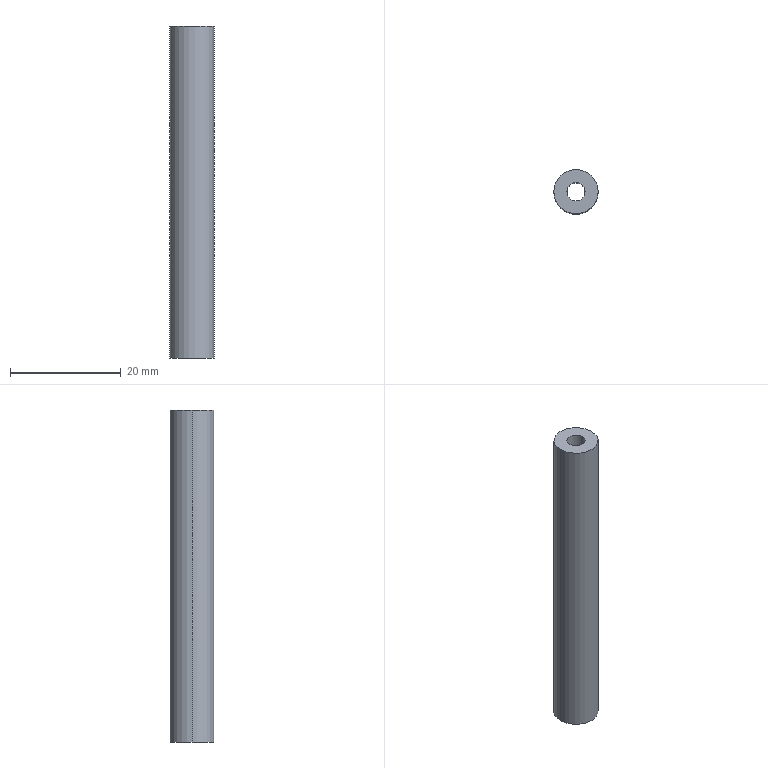Part | SolidWorks | features Extrusion 1 | 1 solid | 6 faces | box 8 x 8 x 60 mm | volume 2503 mm3 | cylinder 4 | plane 2 | commonest cylinder face diameters 3.3 x2 8 x2
STEP:
#1=CARTESIAN_POINT('',(-1.65,0.,-30.));
#2=VERTEX_POINT('',#1);
#3=CARTESIAN_POINT('',(1.65,0.,-30.));
#4=VERTEX_POINT('',#3);
#5=CARTESIAN_POINT('',(0.,0.,-30.));
#6=DIRECTION('',(0.,0.,1.));
#7=DIRECTION('',(1.,0.,0.));
#8=AXIS2_PLACEMENT_3D('',#5,#6,#7);
#9=CIRCLE('',#8,1.65);
#10=EDGE_CURVE('',#2,#4,#9,.T.);
#11=ORIENTED_EDGE('',*,*,#10,.F.);
#12=CARTESIAN_POINT('',(-1.65,0.,30.));
#13=VERTEX_POINT('',#12);
#14=CARTESIAN_POINT('',(-1.65,0.,-30.));
#15=DIRECTION('',(0.,0.,1.));
#16=VECTOR('',#15,1000.);
#17=LINE('',#14,#16);
#18=EDGE_CURVE('',#2,#13,#17,.T.);
#19=ORIENTED_EDGE('',*,*,#18,.T.);
#20=CARTESIAN_POINT('',(1.65,0.,30.));
#21=VERTEX_POINT('',#20);
#22=CARTESIAN_POINT('',(0.,0.,30.));
#23=DIRECTION('',(0.,0.,1.));
#24=DIRECTION('',(1.,0.,0.));
#25=AXIS2_PLACEMENT_3D('',#22,#23,#24);
#26=CIRCLE('',#25,1.65);
#27=EDGE_CURVE('',#13,#21,#26,.T.);
#28=ORIENTED_EDGE('',*,*,#27,.T.);
#29=CARTESIAN_POINT('',(1.65,0.,-30.));
#30=DIRECTION('',(0.,0.,1.));
#31=VECTOR('',#30,1000.);
#32=LINE('',#29,#31);
#33=EDGE_CURVE('',#4,#21,#32,.T.);
#34=ORIENTED_EDGE('',*,*,#33,.F.);
#35=EDGE_LOOP('',(#11,#19,#28,#34));
#36=FACE_OUTER_BOUND('',#35,.T.);
#37=CARTESIAN_POINT('',(0.,0.,-30.));
#38=DIRECTION('',(0.,0.,1.));
#39=DIRECTION('',(1.,0.,0.));
#40=AXIS2_PLACEMENT_3D('',#37,#38,#39);
#41=CYLINDRICAL_SURFACE('',#40,1.65);
#42=ADVANCED_FACE('',(#36),#41,.F.);
#43=CARTESIAN_POINT('',(4.,0.,-30.));
#44=VERTEX_POINT('',#43);
#45=CARTESIAN_POINT('',(-4.,0.,-30.));
#46=VERTEX_POINT('',#45);
#47=CARTESIAN_POINT('',(0.,0.,-30.));
#48=DIRECTION('',(0.,0.,1.));
#49=DIRECTION('',(1.,0.,0.));
#50=AXIS2_PLACEMENT_3D('',#47,#48,#49);
#51=CIRCLE('',#50,4.);
#52=EDGE_CURVE('',#44,#46,#51,.T.);
#53=ORIENTED_EDGE('',*,*,#52,.T.);
#54=CARTESIAN_POINT('',(-4.,0.,30.));
#55=VERTEX_POINT('',#54);
#56=CARTESIAN_POINT('',(-4.,0.,-30.));
#57=DIRECTION('',(0.,0.,1.));
#58=VECTOR('',#57,1000.);
#59=LINE('',#56,#58);
#60=EDGE_CURVE('',#46,#55,#59,.T.);
#61=ORIENTED_EDGE('',*,*,#60,.T.);
#62=CARTESIAN_POINT('',(4.,0.,30.));
#63=VERTEX_POINT('',#62);
#64=CARTESIAN_POINT('',(0.,0.,30.));
#65=DIRECTION('',(0.,0.,1.));
#66=DIRECTION('',(1.,0.,0.));
#67=AXIS2_PLACEMENT_3D('',#64,#65,#66);
#68=CIRCLE('',#67,4.);
#69=EDGE_CURVE('',#63,#55,#68,.T.);
#70=ORIENTED_EDGE('',*,*,#69,.F.);
#71=CARTESIAN_POINT('',(4.,0.,-30.));
#72=DIRECTION('',(0.,0.,1.));
#73=VECTOR('',#72,1000.);
#74=LINE('',#71,#73);
#75=EDGE_CURVE('',#44,#63,#74,.T.);
#76=ORIENTED_EDGE('',*,*,#75,.F.);
#77=EDGE_LOOP('',(#53,#61,#70,#76));
#78=FACE_OUTER_BOUND('',#77,.T.);
#79=CARTESIAN_POINT('',(0.,0.,-30.));
#80=DIRECTION('',(0.,0.,1.));
#81=DIRECTION('',(1.,0.,0.));
#82=AXIS2_PLACEMENT_3D('',#79,#80,#81);
#83=CYLINDRICAL_SURFACE('',#82,4.);
#84=ADVANCED_FACE('',(#78),#83,.T.);
#85=ORIENTED_EDGE('',*,*,#60,.F.);
#86=CARTESIAN_POINT('',(0.,0.,-30.));
#87=DIRECTION('',(0.,0.,1.));
#88=DIRECTION('',(1.,0.,0.));
#89=AXIS2_PLACEMENT_3D('',#86,#87,#88);
#90=CIRCLE('',#89,4.);
#91=EDGE_CURVE('',#46,#44,#90,.T.);
#92=ORIENTED_EDGE('',*,*,#91,.T.);
#93=ORIENTED_EDGE('',*,*,#75,.T.);
#94=CARTESIAN_POINT('',(0.,0.,30.));
#95=DIRECTION('',(0.,0.,1.));
#96=DIRECTION('',(1.,0.,0.));
#97=AXIS2_PLACEMENT_3D('',#94,#95,#96);
#98=CIRCLE('',#97,4.);
#99=EDGE_CURVE('',#55,#63,#98,.T.);
#100=ORIENTED_EDGE('',*,*,#99,.F.);
#101=EDGE_LOOP('',(#85,#92,#93,#100));
#102=FACE_OUTER_BOUND('',#101,.T.);
#103=CARTESIAN_POINT('',(0.,0.,-30.));
#104=DIRECTION('',(0.,0.,1.));
#105=DIRECTION('',(1.,0.,0.));
#106=AXIS2_PLACEMENT_3D('',#103,#104,#105);
#107=CYLINDRICAL_SURFACE('',#106,4.);
#108=ADVANCED_FACE('',(#102),#107,.T.);
#109=CARTESIAN_POINT('',(0.,0.,-30.));
#110=DIRECTION('',(0.,0.,1.));
#111=DIRECTION('',(1.,0.,0.));
#112=AXIS2_PLACEMENT_3D('',#109,#110,#111);
#113=CIRCLE('',#112,1.65);
#114=EDGE_CURVE('',#4,#2,#113,.T.);
#115=ORIENTED_EDGE('',*,*,#114,.T.);
#116=ORIENTED_EDGE('',*,*,#10,.T.);
#117=EDGE_LOOP('',(#115,#116));
#118=FACE_BOUND('',#117,.T.);
#119=ORIENTED_EDGE('',*,*,#52,.F.);
#120=ORIENTED_EDGE('',*,*,#91,.F.);
#121=EDGE_LOOP('',(#119,#120));
#122=FACE_OUTER_BOUND('',#121,.T.);
#123=CARTESIAN_POINT('',(0.,0.,-30.));
#124=DIRECTION('',(0.,0.,1.));
#125=DIRECTION('',(1.,0.,0.));
#126=AXIS2_PLACEMENT_3D('',#123,#124,#125);
#127=PLANE('',#126);
#128=ADVANCED_FACE('',(#118,#122),#127,.F.);
#129=CARTESIAN_POINT('',(0.,0.,30.));
#130=DIRECTION('',(0.,0.,1.));
#131=DIRECTION('',(1.,0.,0.));
#132=AXIS2_PLACEMENT_3D('',#129,#130,#131);
#133=CIRCLE('',#132,1.65);
#134=EDGE_CURVE('',#21,#13,#133,.T.);
#135=ORIENTED_EDGE('',*,*,#134,.F.);
#136=ORIENTED_EDGE('',*,*,#27,.F.);
#137=EDGE_LOOP('',(#135,#136));
#138=FACE_BOUND('',#137,.T.);
#139=ORIENTED_EDGE('',*,*,#69,.T.);
#140=ORIENTED_EDGE('',*,*,#99,.T.);
#141=EDGE_LOOP('',(#139,#140));
#142=FACE_OUTER_BOUND('',#141,.T.);
#143=CARTESIAN_POINT('',(0.,0.,30.));
#144=DIRECTION('',(0.,0.,1.));
#145=DIRECTION('',(1.,0.,0.));
#146=AXIS2_PLACEMENT_3D('',#143,#144,#145);
#147=PLANE('',#146);
#148=ADVANCED_FACE('',(#138,#142),#147,.T.);
#149=ORIENTED_EDGE('',*,*,#18,.F.);
#150=ORIENTED_EDGE('',*,*,#114,.F.);
#151=ORIENTED_EDGE('',*,*,#33,.T.);
#152=ORIENTED_EDGE('',*,*,#134,.T.);
#153=EDGE_LOOP('',(#149,#150,#151,#152));
#154=FACE_OUTER_BOUND('',#153,.T.);
#155=CARTESIAN_POINT('',(0.,0.,-30.));
#156=DIRECTION('',(0.,0.,1.));
#157=DIRECTION('',(1.,0.,0.));
#158=AXIS2_PLACEMENT_3D('',#155,#156,#157);
#159=CYLINDRICAL_SURFACE('',#158,1.65);
#160=ADVANCED_FACE('',(#154),#159,.F.);
#161=CLOSED_SHELL('',(#42,#84,#108,#128,#148,#160));
#162=MANIFOLD_SOLID_BREP('',#161);
#163=CARTESIAN_POINT('',(0.,0.,0.));
#164=DIRECTION('',(0.,0.,1.));
#165=DIRECTION('',(1.,0.,0.));
#166=AXIS2_PLACEMENT_3D('',#163,#164,#165);
#167=(LENGTH_UNIT()NAMED_UNIT(*)SI_UNIT(.MILLI.,.METRE.));
#168=UNCERTAINTY_MEASURE_WITH_UNIT(LENGTH_MEASURE(0.00001),#167,'','');
#169=(NAMED_UNIT(*)PLANE_ANGLE_UNIT()SI_UNIT($,.RADIAN.));
#170=(NAMED_UNIT(*)SI_UNIT($,.STERADIAN.)SOLID_ANGLE_UNIT());
#171=(GEOMETRIC_REPRESENTATION_CONTEXT(3)GLOBAL_UNCERTAINTY_ASSIGNED_CONTEXT((#168))GLOBAL_UNIT_ASSIGNED_CONTEXT((#167,#169,#170))REPRESENTATION_CONTEXT('',''));
#172=ADVANCED_BREP_SHAPE_REPRESENTATION('',(#162,#166),#171);